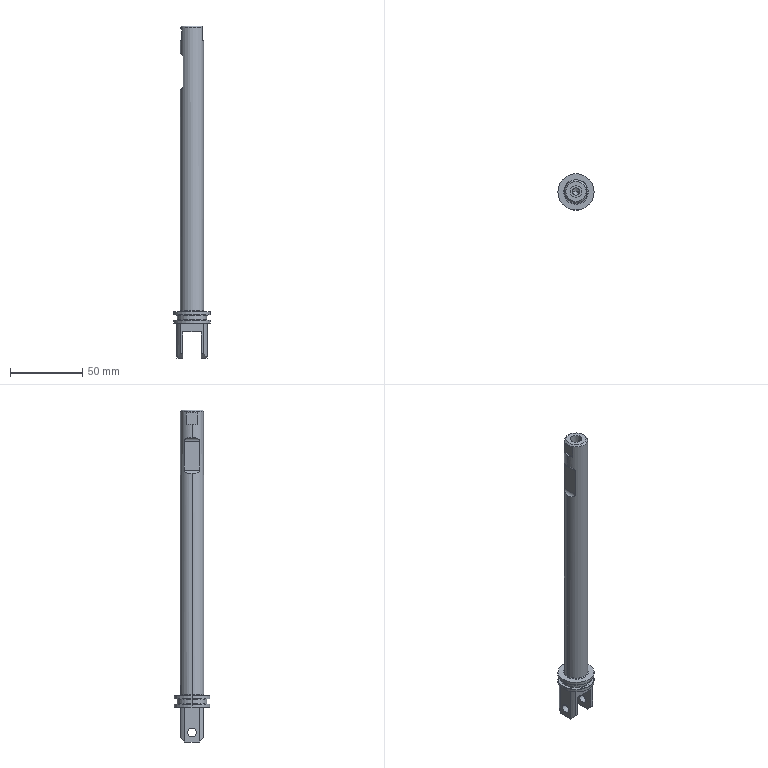Part | SolidWorks | features ICE 7, Fillet 3, HoleWzd 3, Chamfer 1, Extrusion 1, RevCut 1 | 1 solid | 63 faces | box 25 x 25 x 229 mm | volume 45704 mm3 | plane 25 | cylinder 24 | torus 10 | cone 4 | commonest cylinder face diameters 5 x4 6 x4 23 x4 25 x4 2.5 x2 8 x2